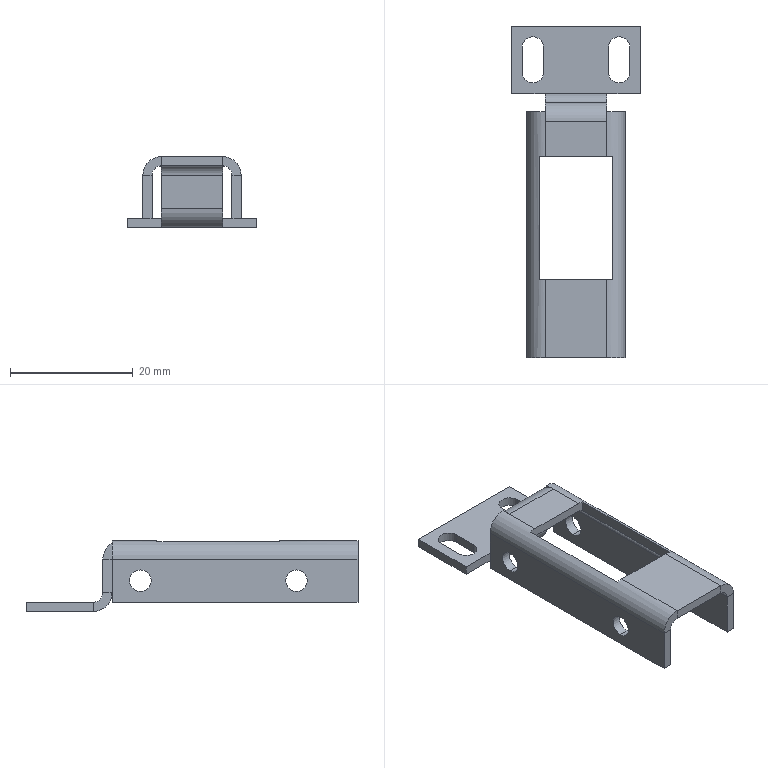Part | STEP file | Cup proximity switch bracket 001 | 1 solid | 64 faces | box 21 x 54 x 11.5 mm | volume 1886 mm3 | plane 44 | cylinder 20 | commonest cylinder face diameters 3.5 x12 3 x4 6 x4